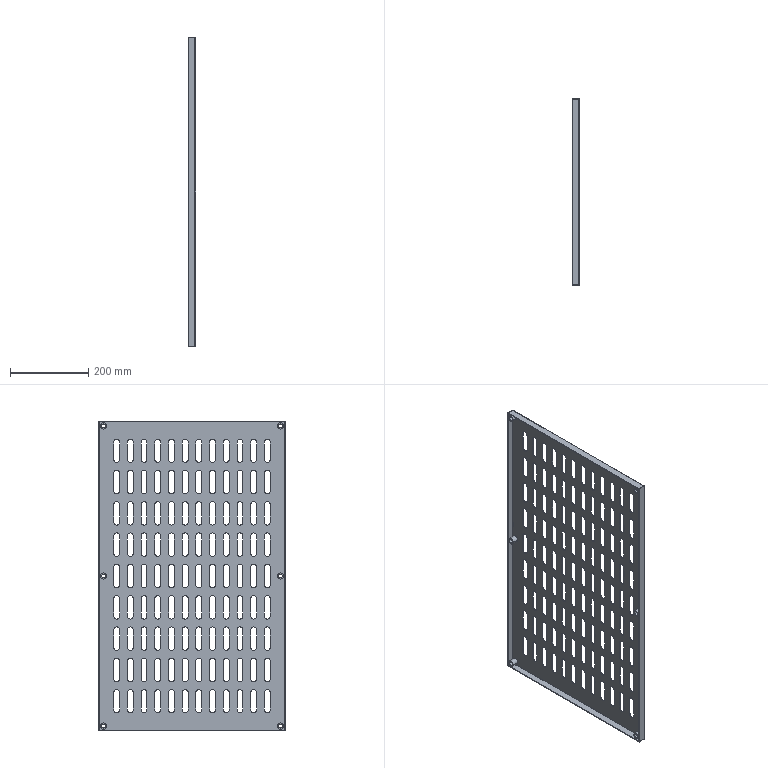Part | SolidWorks | 7 solids | 518 faces | box 19 x 477 x 792 mm | volume 666935 mm3 | cylinder 260 | plane 254 | spline 4 | commonest cylinder face diameters 15 x216 9 x12 10 x12 16 x12 0.2 x4 4.2 x4